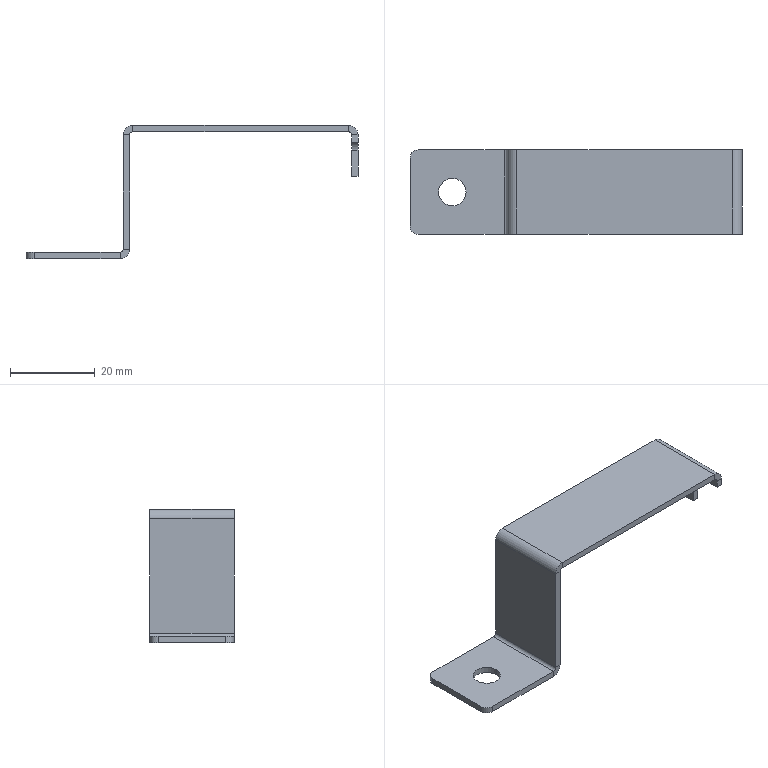Part | STEP file | 10-26 lift limit stopper (Default) | 1 solid | 40 faces | box 78.5 x 20 x 31.5 mm | volume 3271 mm3 | plane 28 | cylinder 12 | commonest cylinder face diameters 4 x4 1.473 x3 4.473 x3 6.5 x2
STEP:
#1=CARTESIAN_POINT('',(-4.75,0.,-1.5));
#2=VERTEX_POINT('',#1);
#3=CARTESIAN_POINT('',(1.75,0.,-1.5));
#4=VERTEX_POINT('',#3);
#5=CARTESIAN_POINT('',(-1.5,0.,-1.5));
#6=DIRECTION('',(0.,0.,1.));
#7=DIRECTION('',(1.,0.,0.));
#8=AXIS2_PLACEMENT_3D('',#5,#6,#7);
#9=CIRCLE('',#8,3.25);
#10=EDGE_CURVE('',#2,#4,#9,.T.);
#11=ORIENTED_EDGE('',*,*,#10,.F.);
#12=CARTESIAN_POINT('',(-4.75,0.,0.));
#13=VERTEX_POINT('',#12);
#14=CARTESIAN_POINT('',(-4.75,0.,-10.));
#15=DIRECTION('',(0.,0.,1.));
#16=VECTOR('',#15,1000.);
#17=LINE('',#14,#16);
#18=EDGE_CURVE('',#2,#13,#17,.T.);
#19=ORIENTED_EDGE('',*,*,#18,.T.);
#20=CARTESIAN_POINT('',(1.75,0.,0.));
#21=VERTEX_POINT('',#20);
#22=CARTESIAN_POINT('',(-1.5,0.,0.));
#23=DIRECTION('',(0.,0.,1.));
#24=DIRECTION('',(1.,0.,0.));
#25=AXIS2_PLACEMENT_3D('',#22,#23,#24);
#26=CIRCLE('',#25,3.25);
#27=EDGE_CURVE('',#13,#21,#26,.T.);
#28=ORIENTED_EDGE('',*,*,#27,.T.);
#29=CARTESIAN_POINT('',(1.75,0.,-10.));
#30=DIRECTION('',(0.,0.,1.));
#31=VECTOR('',#30,1000.);
#32=LINE('',#29,#31);
#33=EDGE_CURVE('',#4,#21,#32,.T.);
#34=ORIENTED_EDGE('',*,*,#33,.F.);
#35=EDGE_LOOP('',(#11,#19,#28,#34));
#36=FACE_OUTER_BOUND('',#35,.T.);
#37=CARTESIAN_POINT('',(-1.5,0.,-10.));
#38=DIRECTION('',(0.,0.,1.));
#39=DIRECTION('',(1.,0.,0.));
#40=AXIS2_PLACEMENT_3D('',#37,#38,#39);
#41=CYLINDRICAL_SURFACE('',#40,3.25);
#42=ADVANCED_FACE('',(#36),#41,.F.);
#43=CARTESIAN_POINT('',(64.763,-10.,28.5));
#44=VERTEX_POINT('',#43);
#45=CARTESIAN_POINT('',(13.737,-10.,28.5));
#46=VERTEX_POINT('',#45);
#47=CARTESIAN_POINT('',(13.,-10.,28.5));
#48=DIRECTION('',(-1.,0.,0.));
#49=VECTOR('',#48,1000.);
#50=LINE('',#47,#49);
#51=EDGE_CURVE('',#44,#46,#50,.T.);
#52=ORIENTED_EDGE('',*,*,#51,.F.);
#53=CARTESIAN_POINT('',(64.763,-10.,30.));
#54=VERTEX_POINT('',#53);
#55=CARTESIAN_POINT('',(64.763,-10.,28.5));
#56=DIRECTION('',(0.,0.,1.));
#57=VECTOR('',#56,1000.);
#58=LINE('',#55,#57);
#59=EDGE_CURVE('',#44,#54,#58,.T.);
#60=ORIENTED_EDGE('',*,*,#59,.T.);
#61=CARTESIAN_POINT('',(13.737,-10.,30.));
#62=VERTEX_POINT('',#61);
#63=CARTESIAN_POINT('',(13.,-10.,30.));
#64=DIRECTION('',(-1.,0.,0.));
#65=VECTOR('',#64,1000.);
#66=LINE('',#63,#65);
#67=EDGE_CURVE('',#54,#62,#66,.T.);
#68=ORIENTED_EDGE('',*,*,#67,.T.);
#69=CARTESIAN_POINT('',(13.737,-10.,28.5));
#70=DIRECTION('',(0.,0.,1.));
#71=VECTOR('',#70,1000.);
#72=LINE('',#69,#71);
#73=EDGE_CURVE('',#46,#62,#72,.T.);
#74=ORIENTED_EDGE('',*,*,#73,.F.);
#75=EDGE_LOOP('',(#52,#60,#68,#74));
#76=FACE_OUTER_BOUND('',#75,.T.);
#77=CARTESIAN_POINT('',(13.,-10.,30.));
#78=DIRECTION('',(0.,-1.,0.));
#79=DIRECTION('',(1.,0.,0.));
#80=AXIS2_PLACEMENT_3D('',#77,#78,#79);
#81=PLANE('',#80);
#82=ADVANCED_FACE('',(#76),#81,.T.);
#83=ORIENTED_EDGE('',*,*,#67,.F.);
#84=CARTESIAN_POINT('',(64.763,10.,30.));
#85=VERTEX_POINT('',#84);
#86=CARTESIAN_POINT('',(64.763,-10.,30.));
#87=DIRECTION('',(0.,1.,0.));
#88=VECTOR('',#87,1000.);
#89=LINE('',#86,#88);
#90=EDGE_CURVE('',#54,#85,#89,.T.);
#91=ORIENTED_EDGE('',*,*,#90,.T.);
#92=CARTESIAN_POINT('',(13.737,10.,30.));
#93=VERTEX_POINT('',#92);
#94=CARTESIAN_POINT('',(65.5,10.,30.));
#95=DIRECTION('',(1.,0.,0.));
#96=VECTOR('',#95,1000.);
#97=LINE('',#94,#96);
#98=EDGE_CURVE('',#93,#85,#97,.T.);
#99=ORIENTED_EDGE('',*,*,#98,.F.);
#100=CARTESIAN_POINT('',(13.737,-10.,30.));
#101=DIRECTION('',(0.,-1.,0.));
#102=VECTOR('',#101,1000.);
#103=LINE('',#100,#102);
#104=EDGE_CURVE('',#93,#62,#103,.T.);
#105=ORIENTED_EDGE('',*,*,#104,.T.);
#106=EDGE_LOOP('',(#83,#91,#99,#105));
#107=FACE_OUTER_BOUND('',#106,.T.);
#108=CARTESIAN_POINT('',(13.,-10.,30.));
#109=DIRECTION('',(0.,0.,1.));
#110=DIRECTION('',(1.,0.,0.));
#111=AXIS2_PLACEMENT_3D('',#108,#109,#110);
#112=PLANE('',#111);
#113=ADVANCED_FACE('',(#107),#112,.T.);
#114=CARTESIAN_POINT('',(64.763,10.,28.5));
#115=VERTEX_POINT('',#114);
#116=CARTESIAN_POINT('',(64.763,-10.,28.5));
#117=DIRECTION('',(0.,1.,0.));
#118=VECTOR('',#117,1000.);
#119=LINE('',#116,#118);
#120=EDGE_CURVE('',#44,#115,#119,.T.);
#121=ORIENTED_EDGE('',*,*,#120,.F.);
#122=ORIENTED_EDGE('',*,*,#51,.T.);
#123=CARTESIAN_POINT('',(13.737,10.,28.5));
#124=VERTEX_POINT('',#123);
#125=CARTESIAN_POINT('',(13.737,10.,28.5));
#126=DIRECTION('',(0.,-1.,0.));
#127=VECTOR('',#126,1000.);
#128=LINE('',#125,#127);
#129=EDGE_CURVE('',#124,#46,#128,.T.);
#130=ORIENTED_EDGE('',*,*,#129,.F.);
#131=CARTESIAN_POINT('',(65.5,10.,28.5));
#132=DIRECTION('',(1.,0.,0.));
#133=VECTOR('',#132,1000.);
#134=LINE('',#131,#133);
#135=EDGE_CURVE('',#124,#115,#134,.T.);
#136=ORIENTED_EDGE('',*,*,#135,.T.);
#137=EDGE_LOOP('',(#121,#122,#130,#136));
#138=FACE_OUTER_BOUND('',#137,.T.);
#139=CARTESIAN_POINT('',(13.,-10.,28.5));
#140=DIRECTION('',(0.,0.,1.));
#141=DIRECTION('',(1.,0.,0.));
#142=AXIS2_PLACEMENT_3D('',#139,#140,#141);
#143=PLANE('',#142);
#144=ADVANCED_FACE('',(#138),#143,.F.);
#145=CARTESIAN_POINT('',(13.,-10.,0.7366));
#146=VERTEX_POINT('',#145);
#147=CARTESIAN_POINT('',(13.,-10.,27.763));
#148=VERTEX_POINT('',#147);
#149=CARTESIAN_POINT('',(13.,-10.,28.5));
#150=DIRECTION('',(0.,0.,1.));
#151=VECTOR('',#150,1000.);
#152=LINE('',#149,#151);
#153=EDGE_CURVE('',#146,#148,#152,.T.);
#154=ORIENTED_EDGE('',*,*,#153,.T.);
#155=CARTESIAN_POINT('',(11.5,-10.,27.763));
#156=VERTEX_POINT('',#155);
#157=CARTESIAN_POINT('',(13.,-10.,27.763));
#158=DIRECTION('',(-1.,0.,0.));
#159=VECTOR('',#158,1000.);
#160=LINE('',#157,#159);
#161=EDGE_CURVE('',#148,#156,#160,.T.);
#162=ORIENTED_EDGE('',*,*,#161,.T.);
#163=CARTESIAN_POINT('',(11.5,-10.,0.7366));
#164=VERTEX_POINT('',#163);
#165=CARTESIAN_POINT('',(11.5,-10.,28.5));
#166=DIRECTION('',(0.,0.,1.));
#167=VECTOR('',#166,1000.);
#168=LINE('',#165,#167);
#169=EDGE_CURVE('',#164,#156,#168,.T.);
#170=ORIENTED_EDGE('',*,*,#169,.F.);
#171=CARTESIAN_POINT('',(11.5,-10.,0.7366));
#172=DIRECTION('',(1.,0.,0.));
#173=VECTOR('',#172,1000.);
#174=LINE('',#171,#173);
#175=EDGE_CURVE('',#164,#146,#174,.T.);
#176=ORIENTED_EDGE('',*,*,#175,.T.);
#177=EDGE_LOOP('',(#154,#162,#170,#176));
#178=FACE_OUTER_BOUND('',#177,.T.);
#179=CARTESIAN_POINT('',(13.,-10.,28.5));
#180=DIRECTION('',(0.,-1.,0.));
#181=DIRECTION('',(1.,0.,0.));
#182=AXIS2_PLACEMENT_3D('',#179,#180,#181);
#183=PLANE('',#182);
#184=ADVANCED_FACE('',(#178),#183,.T.);
#185=CARTESIAN_POINT('',(13.,10.,27.763));
#186=VERTEX_POINT('',#185);
#187=CARTESIAN_POINT('',(13.,10.,0.7366));
#188=VERTEX_POINT('',#187);
#189=CARTESIAN_POINT('',(13.,10.,0.));
#190=DIRECTION('',(0.,0.,-1.));
#191=VECTOR('',#190,1000.);
#192=LINE('',#189,#191);
#193=EDGE_CURVE('',#186,#188,#192,.T.);
#194=ORIENTED_EDGE('',*,*,#193,.F.);
#195=CARTESIAN_POINT('',(13.,-10.,27.763));
#196=DIRECTION('',(0.,1.,0.));
#197=VECTOR('',#196,1000.);
#198=LINE('',#195,#197);
#199=EDGE_CURVE('',#148,#186,#198,.T.);
#200=ORIENTED_EDGE('',*,*,#199,.F.);
#201=ORIENTED_EDGE('',*,*,#153,.F.);
#202=CARTESIAN_POINT('',(13.,10.,0.7366));
#203=DIRECTION('',(0.,1.,0.));
#204=VECTOR('',#203,1000.);
#205=LINE('',#202,#204);
#206=EDGE_CURVE('',#146,#188,#205,.T.);
#207=ORIENTED_EDGE('',*,*,#206,.T.);
#208=EDGE_LOOP('',(#194,#200,#201,#207));
#209=FACE_OUTER_BOUND('',#208,.T.);
#210=CARTESIAN_POINT('',(13.,10.,0.));
#211=DIRECTION('',(1.,0.,0.));
#212=DIRECTION('',(0.,0.,-1.));
#213=AXIS2_PLACEMENT_3D('',#210,#211,#212);
#214=PLANE('',#213);
#215=ADVANCED_FACE('',(#209),#214,.T.);
#216=CARTESIAN_POINT('',(11.5,10.,27.763));
#217=VERTEX_POINT('',#216);
#218=CARTESIAN_POINT('',(11.5,-10.,27.763));
#219=DIRECTION('',(0.,1.,0.));
#220=VECTOR('',#219,1000.);
#221=LINE('',#218,#220);
#222=EDGE_CURVE('',#156,#217,#221,.T.);
#223=ORIENTED_EDGE('',*,*,#222,.T.);
#224=CARTESIAN_POINT('',(11.5,10.,0.7366));
#225=VERTEX_POINT('',#224);
#226=CARTESIAN_POINT('',(11.5,10.,0.));
#227=DIRECTION('',(0.,0.,-1.));
#228=VECTOR('',#227,1000.);
#229=LINE('',#226,#228);
#230=EDGE_CURVE('',#217,#225,#229,.T.);
#231=ORIENTED_EDGE('',*,*,#230,.T.);
#232=CARTESIAN_POINT('',(11.5,-10.,0.7366));
#233=DIRECTION('',(0.,1.,0.));
#234=VECTOR('',#233,1000.);
#235=LINE('',#232,#234);
#236=EDGE_CURVE('',#164,#225,#235,.T.);
#237=ORIENTED_EDGE('',*,*,#236,.F.);
#238=ORIENTED_EDGE('',*,*,#169,.T.);
#239=EDGE_LOOP('',(#223,#231,#237,#238));
#240=FACE_OUTER_BOUND('',#239,.T.);
#241=CARTESIAN_POINT('',(11.5,10.,0.));
#242=DIRECTION('',(1.,0.,0.));
#243=DIRECTION('',(0.,0.,-1.));
#244=AXIS2_PLACEMENT_3D('',#241,#242,#243);
#245=PLANE('',#244);
#246=ADVANCED_FACE('',(#240),#245,.F.);
#247=CARTESIAN_POINT('',(10.763,10.,-1.5));
#248=VERTEX_POINT('',#247);
#249=CARTESIAN_POINT('',(-9.5,10.,-1.5));
#250=VERTEX_POINT('',#249);
#251=CARTESIAN_POINT('',(-11.5,10.,-1.5));
#252=DIRECTION('',(-1.,0.,0.));
#253=VECTOR('',#252,1000.);
#254=LINE('',#251,#253);
#255=EDGE_CURVE('',#248,#250,#254,.T.);
#256=ORIENTED_EDGE('',*,*,#255,.T.);
#257=CARTESIAN_POINT('',(-9.5,10.,0.));
#258=VERTEX_POINT('',#257);
#259=CARTESIAN_POINT('',(-9.5,10.,-1.5));
#260=DIRECTION('',(0.,0.,1.));
#261=VECTOR('',#260,1000.);
#262=LINE('',#259,#261);
#263=EDGE_CURVE('',#250,#258,#262,.T.);
#264=ORIENTED_EDGE('',*,*,#263,.T.);
#265=CARTESIAN_POINT('',(10.763,10.,0.));
#266=VERTEX_POINT('',#265);
#267=CARTESIAN_POINT('',(-11.5,10.,0.));
#268=DIRECTION('',(-1.,0.,0.));
#269=VECTOR('',#268,1000.);
#270=LINE('',#267,#269);
#271=EDGE_CURVE('',#266,#258,#270,.T.);
#272=ORIENTED_EDGE('',*,*,#271,.F.);
#273=CARTESIAN_POINT('',(10.763,10.,0.));
#274=DIRECTION('',(0.,0.,-1.));
#275=VECTOR('',#274,1000.);
#276=LINE('',#273,#275);
#277=EDGE_CURVE('',#266,#248,#276,.T.);
#278=ORIENTED_EDGE('',*,*,#277,.T.);
#279=EDGE_LOOP('',(#256,#264,#272,#278));
#280=FACE_OUTER_BOUND('',#279,.T.);
#281=CARTESIAN_POINT('',(-11.5,10.,-1.5));
#282=DIRECTION('',(0.,1.,0.));
#283=DIRECTION('',(0.,0.,1.));
#284=AXIS2_PLACEMENT_3D('',#281,#282,#283);
#285=PLANE('',#284);
#286=ADVANCED_FACE('',(#280),#285,.T.);
#287=CARTESIAN_POINT('',(-1.5,0.,-1.5));
#288=DIRECTION('',(0.,0.,1.));
#289=DIRECTION('',(1.,0.,0.));
#290=AXIS2_PLACEMENT_3D('',#287,#288,#289);
#291=CIRCLE('',#290,3.25);
#292=EDGE_CURVE('',#4,#2,#291,.T.);
#293=ORIENTED_EDGE('',*,*,#292,.T.);
#294=ORIENTED_EDGE('',*,*,#10,.T.);
#295=EDGE_LOOP('',(#293,#294));
#296=FACE_BOUND('',#295,.T.);
#297=CARTESIAN_POINT('',(-9.5,-10.,-1.5));
#298=VERTEX_POINT('',#297);
#299=CARTESIAN_POINT('',(10.763,-10.,-1.5));
#300=VERTEX_POINT('',#299);
#301=CARTESIAN_POINT('',(-11.5,-10.,-1.5));
#302=DIRECTION('',(1.,0.,0.));
#303=VECTOR('',#302,1000.);
#304=LINE('',#301,#303);
#305=EDGE_CURVE('',#298,#300,#304,.T.);
#306=ORIENTED_EDGE('',*,*,#305,.F.);
#307=CARTESIAN_POINT('',(-11.5,-8.,-1.5));
#308=VERTEX_POINT('',#307);
#309=CARTESIAN_POINT('',(-9.5,-8.,-1.5));
#310=DIRECTION('',(0.,0.,-1.));
#311=DIRECTION('',(1.,0.,0.));
#312=AXIS2_PLACEMENT_3D('',#309,#310,#311);
#313=CIRCLE('',#312,2.);
#314=EDGE_CURVE('',#298,#308,#313,.T.);
#315=ORIENTED_EDGE('',*,*,#314,.T.);
#316=CARTESIAN_POINT('',(-11.5,8.,-1.5));
#317=VERTEX_POINT('',#316);
#318=CARTESIAN_POINT('',(-11.5,10.,-1.5));
#319=DIRECTION('',(0.,-1.,0.));
#320=VECTOR('',#319,1000.);
#321=LINE('',#318,#320);
#322=EDGE_CURVE('',#317,#308,#321,.T.);
#323=ORIENTED_EDGE('',*,*,#322,.F.);
#324=CARTESIAN_POINT('',(-9.5,8.,-1.5));
#325=DIRECTION('',(0.,0.,-1.));
#326=DIRECTION('',(1.,0.,0.));
#327=AXIS2_PLACEMENT_3D('',#324,#325,#326);
#328=CIRCLE('',#327,2.);
#329=EDGE_CURVE('',#317,#250,#328,.T.);
#330=ORIENTED_EDGE('',*,*,#329,.T.);
#331=ORIENTED_EDGE('',*,*,#255,.F.);
#332=CARTESIAN_POINT('',(10.763,10.,-1.5));
#333=DIRECTION('',(0.,-1.,0.));
#334=VECTOR('',#333,1000.);
#335=LINE('',#332,#334);
#336=EDGE_CURVE('',#248,#300,#335,.T.);
#337=ORIENTED_EDGE('',*,*,#336,.T.);
#338=EDGE_LOOP('',(#306,#315,#323,#330,#331,#337));
#339=FACE_OUTER_BOUND('',#338,.T.);
#340=CARTESIAN_POINT('',(11.5,-10.,-1.5));
#341=DIRECTION('',(0.,0.,1.));
#342=DIRECTION('',(1.,0.,0.));
#343=AXIS2_PLACEMENT_3D('',#340,#341,#342);
#344=PLANE('',#343);
#345=ADVANCED_FACE('',(#296,#339),#344,.F.);
#346=CARTESIAN_POINT('',(-1.5,0.,0.));
#347=DIRECTION('',(0.,0.,1.));
#348=DIRECTION('',(1.,0.,0.));
#349=AXIS2_PLACEMENT_3D('',#346,#347,#348);
#350=CIRCLE('',#349,3.25);
#351=EDGE_CURVE('',#21,#13,#350,.T.);
#352=ORIENTED_EDGE('',*,*,#351,.F.);
#353=ORIENTED_EDGE('',*,*,#27,.F.);
#354=EDGE_LOOP('',(#352,#353));
#355=FACE_BOUND('',#354,.T.);
#356=CARTESIAN_POINT('',(-11.5,8.,0.));
#357=VERTEX_POINT('',#356);
#358=CARTESIAN_POINT('',(-11.5,-8.,0.));
#359=VERTEX_POINT('',#358);
#360=CARTESIAN_POINT('',(-11.5,10.,0.));
#361=DIRECTION('',(0.,-1.,0.));
#362=VECTOR('',#361,1000.);
#363=LINE('',#360,#362);
#364=EDGE_CURVE('',#357,#359,#363,.T.);
#365=ORIENTED_EDGE('',*,*,#364,.T.);
#366=CARTESIAN_POINT('',(-9.5,-10.,0.));
#367=VERTEX_POINT('',#366);
#368=CARTESIAN_POINT('',(-9.5,-8.,0.));
#369=DIRECTION('',(0.,0.,1.));
#370=DIRECTION('',(1.,0.,0.));
#371=AXIS2_PLACEMENT_3D('',#368,#369,#370);
#372=CIRCLE('',#371,2.);
#373=EDGE_CURVE('',#359,#367,#372,.T.);
#374=ORIENTED_EDGE('',*,*,#373,.T.);
#375=CARTESIAN_POINT('',(10.763,-10.,0.));
#376=VERTEX_POINT('',#375);
#377=CARTESIAN_POINT('',(-11.5,-10.,0.));
#378=DIRECTION('',(1.,0.,0.));
#379=VECTOR('',#378,1000.);
#380=LINE('',#377,#379);
#381=EDGE_CURVE('',#367,#376,#380,.T.);
#382=ORIENTED_EDGE('',*,*,#381,.T.);
#383=CARTESIAN_POINT('',(10.763,10.,0.));
#384=DIRECTION('',(0.,-1.,0.));
#385=VECTOR('',#384,1000.);
#386=LINE('',#383,#385);
#387=EDGE_CURVE('',#266,#376,#386,.T.);
#388=ORIENTED_EDGE('',*,*,#387,.F.);
#389=ORIENTED_EDGE('',*,*,#271,.T.);
#390=CARTESIAN_POINT('',(-9.5,8.,0.));
#391=DIRECTION('',(0.,0.,1.));
#392=DIRECTION('',(1.,0.,0.));
#393=AXIS2_PLACEMENT_3D('',#390,#391,#392);
#394=CIRCLE('',#393,2.);
#395=EDGE_CURVE('',#258,#357,#394,.T.);
#396=ORIENTED_EDGE('',*,*,#395,.T.);
#397=EDGE_LOOP('',(#365,#374,#382,#388,#389,#396));
#398=FACE_OUTER_BOUND('',#397,.T.);
#399=CARTESIAN_POINT('',(11.5,-10.,0.));
#400=DIRECTION('',(0.,0.,1.));
#401=DIRECTION('',(1.,0.,0.));
#402=AXIS2_PLACEMENT_3D('',#399,#400,#401);
#403=PLANE('',#402);
#404=ADVANCED_FACE('',(#355,#398),#403,.T.);
#405=ORIENTED_EDGE('',*,*,#381,.F.);
#406=CARTESIAN_POINT('',(-9.5,-10.,-1.5));
#407=DIRECTION('',(0.,0.,-1.));
#408=VECTOR('',#407,1000.);
#409=LINE('',#406,#408);
#410=EDGE_CURVE('',#367,#298,#409,.T.);
#411=ORIENTED_EDGE('',*,*,#410,.T.);
#412=ORIENTED_EDGE('',*,*,#305,.T.);
#413=CARTESIAN_POINT('',(10.763,-10.,0.));
#414=DIRECTION('',(0.,0.,-1.));
#415=VECTOR('',#414,1000.);
#416=LINE('',#413,#415);
#417=EDGE_CURVE('',#376,#300,#416,.T.);
#418=ORIENTED_EDGE('',*,*,#417,.F.);
#419=EDGE_LOOP('',(#405,#411,#412,#418));
#420=FACE_OUTER_BOUND('',#419,.T.);
#421=CARTESIAN_POINT('',(-11.5,-10.,-1.5));
#422=DIRECTION('',(0.,-1.,0.));
#423=DIRECTION('',(0.,0.,-1.));
#424=AXIS2_PLACEMENT_3D('',#421,#422,#423);
#425=PLANE('',#424);
#426=ADVANCED_FACE('',(#420),#425,.T.);
#427=ORIENTED_EDGE('',*,*,#322,.T.);
#428=CARTESIAN_POINT('',(-11.5,-8.,-1.5));
#429=DIRECTION('',(0.,0.,1.));
#430=VECTOR('',#429,1000.);
#431=LINE('',#428,#430);
#432=EDGE_CURVE('',#308,#359,#431,.T.);
#433=ORIENTED_EDGE('',*,*,#432,.T.);
#434=ORIENTED_EDGE('',*,*,#364,.F.);
#435=CARTESIAN_POINT('',(-11.5,8.,-1.5));
#436=DIRECTION('',(0.,0.,-1.));
#437=VECTOR('',#436,1000.);
#438=LINE('',#435,#437);
#439=EDGE_CURVE('',#357,#317,#438,.T.);
#440=ORIENTED_EDGE('',*,*,#439,.T.);
#441=EDGE_LOOP('',(#427,#433,#434,#440));
#442=FACE_OUTER_BOUND('',#441,.T.);
#443=CARTESIAN_POINT('',(-11.5,10.,-1.5));
#444=DIRECTION('',(-1.,0.,0.));
#445=DIRECTION('',(0.,0.,1.));
#446=AXIS2_PLACEMENT_3D('',#443,#444,#445);
#447=PLANE('',#446);
#448=ADVANCED_FACE('',(#442),#447,.T.);
#449=ORIENTED_EDGE('',*,*,#175,.F.);
#450=CARTESIAN_POINT('',(10.763,-10.,0.7366));
#451=DIRECTION('',(0.,-1.,0.));
#452=DIRECTION('',(0.,0.,1.));
#453=AXIS2_PLACEMENT_3D('',#450,#451,#452);
#454=CIRCLE('',#453,0.7366);
#455=EDGE_CURVE('',#376,#164,#454,.T.);
#456=ORIENTED_EDGE('',*,*,#455,.F.);
#457=ORIENTED_EDGE('',*,*,#417,.T.);
#458=CARTESIAN_POINT('',(10.763,-10.,0.7366));
#459=DIRECTION('',(0.,-1.,0.));
#460=DIRECTION('',(0.,0.,1.));
#461=AXIS2_PLACEMENT_3D('',#458,#459,#460);
#462=CIRCLE('',#461,2.237);
#463=EDGE_CURVE('',#300,#146,#462,.T.);
#464=ORIENTED_EDGE('',*,*,#463,.T.);
#465=EDGE_LOOP('',(#449,#456,#457,#464));
#466=FACE_OUTER_BOUND('',#465,.T.);
#467=CARTESIAN_POINT('',(10.763,-10.,0.7366));
#468=DIRECTION('',(0.,-1.,0.));
#469=DIRECTION('',(0.,0.,-1.));
#470=AXIS2_PLACEMENT_3D('',#467,#468,#469);
#471=PLANE('',#470);
#472=ADVANCED_FACE('',(#466),#471,.T.);
#473=CARTESIAN_POINT('',(10.763,10.,0.7366));
#474=DIRECTION('',(0.,1.,0.));
#475=DIRECTION('',(0.,0.,1.));
#476=AXIS2_PLACEMENT_3D('',#473,#474,#475);
#477=CIRCLE('',#476,0.7366);
#478=EDGE_CURVE('',#225,#266,#477,.T.);
#479=ORIENTED_EDGE('',*,*,#478,.F.);
#480=CARTESIAN_POINT('',(11.5,10.,0.7366));
#481=DIRECTION('',(1.,0.,0.));
#482=VECTOR('',#481,1000.);
#483=LINE('',#480,#482);
#484=EDGE_CURVE('',#225,#188,#483,.T.);
#485=ORIENTED_EDGE('',*,*,#484,.T.);
#486=CARTESIAN_POINT('',(10.763,10.,0.7366));
#487=DIRECTION('',(0.,1.,0.));
#488=DIRECTION('',(0.,0.,1.));
#489=AXIS2_PLACEMENT_3D('',#486,#487,#488);
#490=CIRCLE('',#489,2.237);
#491=EDGE_CURVE('',#188,#248,#490,.T.);
#492=ORIENTED_EDGE('',*,*,#491,.T.);
#493=ORIENTED_EDGE('',*,*,#277,.F.);
#494=EDGE_LOOP('',(#479,#485,#492,#493));
#495=FACE_OUTER_BOUND('',#494,.T.);
#496=CARTESIAN_POINT('',(10.763,10.,0.7366));
#497=DIRECTION('',(0.,-1.,0.));
#498=DIRECTION('',(0.,0.,-1.));
#499=AXIS2_PLACEMENT_3D('',#496,#497,#498);
#500=PLANE('',#499);
#501=ADVANCED_FACE('',(#495),#500,.F.);
#502=ORIENTED_EDGE('',*,*,#336,.F.);
#503=ORIENTED_EDGE('',*,*,#491,.F.);
#504=ORIENTED_EDGE('',*,*,#206,.F.);
#505=ORIENTED_EDGE('',*,*,#463,.F.);
#506=EDGE_LOOP('',(#502,#503,#504,#505));
#507=FACE_OUTER_BOUND('',#506,.T.);
#508=CARTESIAN_POINT('',(10.763,10.,0.7366));
#509=DIRECTION('',(0.,1.,0.));
#510=DIRECTION('',(1.,0.,0.));
#511=AXIS2_PLACEMENT_3D('',#508,#509,#510);
#512=CYLINDRICAL_SURFACE('',#511,2.237);
#513=ADVANCED_FACE('',(#507),#512,.T.);
#514=ORIENTED_EDGE('',*,*,#387,.T.);
#515=ORIENTED_EDGE('',*,*,#455,.T.);
#516=ORIENTED_EDGE('',*,*,#236,.T.);
#517=ORIENTED_EDGE('',*,*,#478,.T.);
#518=EDGE_LOOP('',(#514,#515,#516,#517));
#519=FACE_OUTER_BOUND('',#518,.T.);
#520=CARTESIAN_POINT('',(10.763,10.,0.7366));
#521=DIRECTION('',(0.,1.,0.));
#522=DIRECTION('',(1.,0.,0.));
#523=AXIS2_PLACEMENT_3D('',#520,#521,#522);
#524=CYLINDRICAL_SURFACE('',#523,0.7366);
#525=ADVANCED_FACE('',(#519),#524,.F.);
#526=CARTESIAN_POINT('',(13.,10.,27.763));
#527=DIRECTION('',(-1.,0.,0.));
#528=VECTOR('',#527,1000.);
#529=LINE('',#526,#528);
#530=EDGE_CURVE('',#186,#217,#529,.T.);
#531=ORIENTED_EDGE('',*,*,#530,.F.);
#532=ORIENTED_EDGE('',*,*,#193,.T.);
#533=ORIENTED_EDGE('',*,*,#484,.F.);
#534=ORIENTED_EDGE('',*,*,#230,.F.);
#535=EDGE_LOOP('',(#531,#532,#533,#534));
#536=FACE_OUTER_BOUND('',#535,.T.);
#537=CARTESIAN_POINT('',(13.,10.,0.));
#538=DIRECTION('',(0.,1.,0.));
#539=DIRECTION('',(-1.,0.,0.));
#540=AXIS2_PLACEMENT_3D('',#537,#538,#539);
#541=PLANE('',#540);
#542=ADVANCED_FACE('',(#536),#541,.T.);
#543=CARTESIAN_POINT('',(13.737,10.,28.5));
#544=DIRECTION('',(0.,0.,1.));
#545=VECTOR('',#544,1000.);
#546=LINE('',#543,#545);
#547=EDGE_CURVE('',#124,#93,#546,.T.);
#548=ORIENTED_EDGE('',*,*,#547,.F.);
#549=CARTESIAN_POINT('',(13.737,10.,27.763));
#550=DIRECTION('',(0.,1.,0.));
#551=DIRECTION('',(0.,0.,-1.));
#552=AXIS2_PLACEMENT_3D('',#549,#550,#551);
#553=CIRCLE('',#552,0.7366);
#554=EDGE_CURVE('',#186,#124,#553,.T.);
#555=ORIENTED_EDGE('',*,*,#554,.F.);
#556=ORIENTED_EDGE('',*,*,#530,.T.);
#557=CARTESIAN_POINT('',(13.737,10.,27.763));
#558=DIRECTION('',(0.,1.,0.));
#559=DIRECTION('',(0.,0.,-1.));
#560=AXIS2_PLACEMENT_3D('',#557,#558,#559);
#561=CIRCLE('',#560,2.237);
#562=EDGE_CURVE('',#217,#93,#561,.T.);
#563=ORIENTED_EDGE('',*,*,#562,.T.);
#564=EDGE_LOOP('',(#548,#555,#556,#563));
#565=FACE_OUTER_BOUND('',#564,.T.);
#566=CARTESIAN_POINT('',(13.737,10.,27.763));
#567=DIRECTION('',(0.,1.,0.));
#568=DIRECTION('',(0.,0.,1.));
#569=AXIS2_PLACEMENT_3D('',#566,#567,#568);
#570=PLANE('',#569);
#571=ADVANCED_FACE('',(#565),#570,.T.);
#572=CARTESIAN_POINT('',(13.737,-10.,27.763));
#573=DIRECTION('',(0.,-1.,0.));
#574=DIRECTION('',(0.,0.,-1.));
#575=AXIS2_PLACEMENT_3D('',#572,#573,#574);
#576=CIRCLE('',#575,0.7366);
#577=EDGE_CURVE('',#46,#148,#576,.T.);
#578=ORIENTED_EDGE('',*,*,#577,.F.);
#579=ORIENTED_EDGE('',*,*,#73,.T.);
#580=CARTESIAN_POINT('',(13.737,-10.,27.763));
#581=DIRECTION('',(0.,-1.,0.));
#582=DIRECTION('',(0.,0.,-1.));
#583=AXIS2_PLACEMENT_3D('',#580,#581,#582);
#584=CIRCLE('',#583,2.237);
#585=EDGE_CURVE('',#62,#156,#584,.T.);
#586=ORIENTED_EDGE('',*,*,#585,.T.);
#587=ORIENTED_EDGE('',*,*,#161,.F.);
#588=EDGE_LOOP('',(#578,#579,#586,#587));
#589=FACE_OUTER_BOUND('',#588,.T.);
#590=CARTESIAN_POINT('',(13.737,-10.,27.763));
#591=DIRECTION('',(0.,1.,0.));
#592=DIRECTION('',(0.,0.,1.));
#593=AXIS2_PLACEMENT_3D('',#590,#591,#592);
#594=PLANE('',#593);
#595=ADVANCED_FACE('',(#589),#594,.F.);
#596=ORIENTED_EDGE('',*,*,#222,.F.);
#597=ORIENTED_EDGE('',*,*,#585,.F.);
#598=ORIENTED_EDGE('',*,*,#104,.F.);
#599=ORIENTED_EDGE('',*,*,#562,.F.);
#600=EDGE_LOOP('',(#596,#597,#598,#599));
#601=FACE_OUTER_BOUND('',#600,.T.);
#602=CARTESIAN_POINT('',(13.737,-10.,27.763));
#603=DIRECTION('',(0.,-1.,0.));
#604=DIRECTION('',(0.,0.,1.));
#605=AXIS2_PLACEMENT_3D('',#602,#603,#604);
#606=CYLINDRICAL_SURFACE('',#605,2.237);
#607=ADVANCED_FACE('',(#601),#606,.T.);
#608=ORIENTED_EDGE('',*,*,#199,.T.);
#609=ORIENTED_EDGE('',*,*,#554,.T.);
#610=ORIENTED_EDGE('',*,*,#129,.T.);
#611=ORIENTED_EDGE('',*,*,#577,.T.);
#612=EDGE_LOOP('',(#608,#609,#610,#611));
#613=FACE_OUTER_BOUND('',#612,.T.);
#614=CARTESIAN_POINT('',(13.737,-10.,27.763));
#615=DIRECTION('',(0.,-1.,0.));
#616=DIRECTION('',(0.,0.,1.));
#617=AXIS2_PLACEMENT_3D('',#614,#615,#616);
#618=CYLINDRICAL_SURFACE('',#617,0.7366);
#619=ADVANCED_FACE('',(#613),#618,.F.);
#620=CARTESIAN_POINT('',(64.763,10.,28.5));
#621=DIRECTION('',(0.,0.,1.));
#622=VECTOR('',#621,1000.);
#623=LINE('',#620,#622);
#624=EDGE_CURVE('',#115,#85,#623,.T.);
#625=ORIENTED_EDGE('',*,*,#624,.F.);
#626=ORIENTED_EDGE('',*,*,#135,.F.);
#627=ORIENTED_EDGE('',*,*,#547,.T.);
#628=ORIENTED_EDGE('',*,*,#98,.T.);
#629=EDGE_LOOP('',(#625,#626,#627,#628));
#630=FACE_OUTER_BOUND('',#629,.T.);
#631=CARTESIAN_POINT('',(65.5,10.,30.));
#632=DIRECTION('',(0.,1.,0.));
#633=DIRECTION('',(-1.,0.,0.));
#634=AXIS2_PLACEMENT_3D('',#631,#632,#633);
#635=PLANE('',#634);
#636=ADVANCED_FACE('',(#630),#635,.T.);
#637=CARTESIAN_POINT('',(65.5,10.,27.763));
#638=VERTEX_POINT('',#637);
#639=CARTESIAN_POINT('',(67.,10.,27.763));
#640=VERTEX_POINT('',#639);
#641=CARTESIAN_POINT('',(65.5,10.,27.763));
#642=DIRECTION('',(1.,0.,0.));
#643=VECTOR('',#642,1000.);
#644=LINE('',#641,#643);
#645=EDGE_CURVE('',#638,#640,#644,.T.);
#646=ORIENTED_EDGE('',*,*,#645,.F.);
#647=CARTESIAN_POINT('',(64.763,10.,27.763));
#648=DIRECTION('',(0.,1.,0.));
#649=DIRECTION('',(0.,0.,-1.));
#650=AXIS2_PLACEMENT_3D('',#647,#648,#649);
#651=CIRCLE('',#650,0.7366);
#652=EDGE_CURVE('',#115,#638,#651,.T.);
#653=ORIENTED_EDGE('',*,*,#652,.F.);
#654=ORIENTED_EDGE('',*,*,#624,.T.);
#655=CARTESIAN_POINT('',(64.763,10.,27.763));
#656=DIRECTION('',(0.,1.,0.));
#657=DIRECTION('',(0.,0.,-1.));
#658=AXIS2_PLACEMENT_3D('',#655,#656,#657);
#659=CIRCLE('',#658,2.237);
#660=EDGE_CURVE('',#85,#640,#659,.T.);
#661=ORIENTED_EDGE('',*,*,#660,.T.);
#662=EDGE_LOOP('',(#646,#653,#654,#661));
#663=FACE_OUTER_BOUND('',#662,.T.);
#664=CARTESIAN_POINT('',(64.763,10.,27.763));
#665=DIRECTION('',(0.,1.,0.));
#666=DIRECTION('',(0.,0.,1.));
#667=AXIS2_PLACEMENT_3D('',#664,#665,#666);
#668=PLANE('',#667);
#669=ADVANCED_FACE('',(#663),#668,.T.);
#670=CARTESIAN_POINT('',(65.5,-10.,27.763));
#671=VERTEX_POINT('',#670);
#672=CARTESIAN_POINT('',(64.763,-10.,27.763));
#673=DIRECTION('',(0.,-1.,0.));
#674=DIRECTION('',(0.,0.,-1.));
#675=AXIS2_PLACEMENT_3D('',#672,#673,#674);
#676=CIRCLE('',#675,0.7366);
#677=EDGE_CURVE('',#671,#44,#676,.T.);
#678=ORIENTED_EDGE('',*,*,#677,.F.);
#679=CARTESIAN_POINT('',(67.,-10.,27.763));
#680=VERTEX_POINT('',#679);
#681=CARTESIAN_POINT('',(65.5,-10.,27.763));
#682=DIRECTION('',(1.,0.,0.));
#683=VECTOR('',#682,1000.);
#684=LINE('',#681,#683);
#685=EDGE_CURVE('',#671,#680,#684,.T.);
#686=ORIENTED_EDGE('',*,*,#685,.T.);
#687=CARTESIAN_POINT('',(64.763,-10.,27.763));
#688=DIRECTION('',(0.,-1.,0.));
#689=DIRECTION('',(0.,0.,-1.));
#690=AXIS2_PLACEMENT_3D('',#687,#688,#689);
#691=CIRCLE('',#690,2.237);
#692=EDGE_CURVE('',#680,#54,#691,.T.);
#693=ORIENTED_EDGE('',*,*,#692,.T.);
#694=ORIENTED_EDGE('',*,*,#59,.F.);
#695=EDGE_LOOP('',(#678,#686,#693,#694));
#696=FACE_OUTER_BOUND('',#695,.T.);
#697=CARTESIAN_POINT('',(64.763,-10.,27.763));
#698=DIRECTION('',(0.,1.,0.));
#699=DIRECTION('',(0.,0.,1.));
#700=AXIS2_PLACEMENT_3D('',#697,#698,#699);
#701=PLANE('',#700);
#702=ADVANCED_FACE('',(#696),#701,.F.);
#703=ORIENTED_EDGE('',*,*,#90,.F.);
#704=ORIENTED_EDGE('',*,*,#692,.F.);
#705=CARTESIAN_POINT('',(67.,-10.,27.763));
#706=DIRECTION('',(0.,-1.,0.));
#707=VECTOR('',#706,1000.);
#708=LINE('',#705,#707);
#709=EDGE_CURVE('',#640,#680,#708,.T.);
#710=ORIENTED_EDGE('',*,*,#709,.F.);
#711=ORIENTED_EDGE('',*,*,#660,.F.);
#712=EDGE_LOOP('',(#703,#704,#710,#711));
#713=FACE_OUTER_BOUND('',#712,.T.);
#714=CARTESIAN_POINT('',(64.763,-10.,27.763));
#715=DIRECTION('',(0.,-1.,0.));
#716=DIRECTION('',(1.,0.,0.));
#717=AXIS2_PLACEMENT_3D('',#714,#715,#716);
#718=CYLINDRICAL_SURFACE('',#717,2.237);
#719=ADVANCED_FACE('',(#713),#718,.T.);
#720=ORIENTED_EDGE('',*,*,#120,.T.);
#721=ORIENTED_EDGE('',*,*,#652,.T.);
#722=CARTESIAN_POINT('',(65.5,10.,27.763));
#723=DIRECTION('',(0.,-1.,0.));
#724=VECTOR('',#723,1000.);
#725=LINE('',#722,#724);
#726=EDGE_CURVE('',#638,#671,#725,.T.);
#727=ORIENTED_EDGE('',*,*,#726,.T.);
#728=ORIENTED_EDGE('',*,*,#677,.T.);
#729=EDGE_LOOP('',(#720,#721,#727,#728));
#730=FACE_OUTER_BOUND('',#729,.T.);
#731=CARTESIAN_POINT('',(64.763,-10.,27.763));
#732=DIRECTION('',(0.,-1.,0.));
#733=DIRECTION('',(1.,0.,0.));
#734=AXIS2_PLACEMENT_3D('',#731,#732,#733);
#735=CYLINDRICAL_SURFACE('',#734,0.7366);
#736=ADVANCED_FACE('',(#730),#735,.F.);
#737=CARTESIAN_POINT('',(65.5,-10.,26.));
#738=VERTEX_POINT('',#737);
#739=CARTESIAN_POINT('',(67.,-10.,26.));
#740=VERTEX_POINT('',#739);
#741=CARTESIAN_POINT('',(57.,-10.,26.));
#742=DIRECTION('',(1.,0.,0.));
#743=VECTOR('',#742,1000.);
#744=LINE('',#741,#743);
#745=EDGE_CURVE('',#738,#740,#744,.T.);
#746=ORIENTED_EDGE('',*,*,#745,.T.);
#747=CARTESIAN_POINT('',(67.,-10.,28.5));
#748=DIRECTION('',(0.,0.,1.));
#749=VECTOR('',#748,1000.);
#750=LINE('',#747,#749);
#751=EDGE_CURVE('',#740,#680,#750,.T.);
#752=ORIENTED_EDGE('',*,*,#751,.T.);
#753=ORIENTED_EDGE('',*,*,#685,.F.);
#754=CARTESIAN_POINT('',(65.5,-10.,28.5));
#755=DIRECTION('',(0.,0.,1.));
#756=VECTOR('',#755,1000.);
#757=LINE('',#754,#756);
#758=EDGE_CURVE('',#738,#671,#757,.T.);
#759=ORIENTED_EDGE('',*,*,#758,.F.);
#760=EDGE_LOOP('',(#746,#752,#753,#759));
#761=FACE_OUTER_BOUND('',#760,.T.);
#762=CARTESIAN_POINT('',(67.,-10.,28.5));
#763=DIRECTION('',(0.,-1.,0.));
#764=DIRECTION('',(0.,0.,-1.));
#765=AXIS2_PLACEMENT_3D('',#762,#763,#764);
#766=PLANE('',#765);
#767=ADVANCED_FACE('',(#761),#766,.T.);
#768=CARTESIAN_POINT('',(65.5,10.,26.));
#769=VERTEX_POINT('',#768);
#770=CARTESIAN_POINT('',(67.,10.,26.));
#771=VERTEX_POINT('',#770);
#772=CARTESIAN_POINT('',(57.,10.,26.));
#773=DIRECTION('',(1.,0.,0.));
#774=VECTOR('',#773,1000.);
#775=LINE('',#772,#774);
#776=EDGE_CURVE('',#769,#771,#775,.T.);
#777=ORIENTED_EDGE('',*,*,#776,.F.);
#778=CARTESIAN_POINT('',(65.5,10.,18.));
#779=DIRECTION('',(0.,0.,-1.));
#780=VECTOR('',#779,1000.);
#781=LINE('',#778,#780);
#782=EDGE_CURVE('',#638,#769,#781,.T.);
#783=ORIENTED_EDGE('',*,*,#782,.F.);
#784=ORIENTED_EDGE('',*,*,#645,.T.);
#785=CARTESIAN_POINT('',(67.,10.,18.));
#786=DIRECTION('',(0.,0.,-1.));
#787=VECTOR('',#786,1000.);
#788=LINE('',#785,#787);
#789=EDGE_CURVE('',#640,#771,#788,.T.);
#790=ORIENTED_EDGE('',*,*,#789,.T.);
#791=EDGE_LOOP('',(#777,#783,#784,#790));
#792=FACE_OUTER_BOUND('',#791,.T.);
#793=CARTESIAN_POINT('',(67.,10.,18.));
#794=DIRECTION('',(0.,1.,0.));
#795=DIRECTION('',(0.,0.,1.));
#796=AXIS2_PLACEMENT_3D('',#793,#794,#795);
#797=PLANE('',#796);
#798=ADVANCED_FACE('',(#792),#797,.T.);
#799=CARTESIAN_POINT('',(67.,-4.,26.));
#800=VERTEX_POINT('',#799);
#801=CARTESIAN_POINT('',(67.,-2.,26.));
#802=DIRECTION('',(0.,-1.,0.));
#803=VECTOR('',#802,1000.);
#804=LINE('',#801,#803);
#805=EDGE_CURVE('',#800,#740,#804,.T.);
#806=ORIENTED_EDGE('',*,*,#805,.F.);
#807=CARTESIAN_POINT('',(67.,-2.,24.));
#808=VERTEX_POINT('',#807);
#809=CARTESIAN_POINT('',(67.,-4.,24.));
#810=DIRECTION('',(-1.,0.,0.));
#811=DIRECTION('',(0.,0.,-1.));
#812=AXIS2_PLACEMENT_3D('',#809,#810,#811);
#813=CIRCLE('',#812,2.);
#814=EDGE_CURVE('',#800,#808,#813,.T.);
#815=ORIENTED_EDGE('',*,*,#814,.T.);
#816=CARTESIAN_POINT('',(67.,-2.,18.));
#817=VERTEX_POINT('',#816);
#818=CARTESIAN_POINT('',(67.,-2.,18.));
#819=DIRECTION('',(0.,0.,1.));
#820=VECTOR('',#819,1000.);
#821=LINE('',#818,#820);
#822=EDGE_CURVE('',#817,#808,#821,.T.);
#823=ORIENTED_EDGE('',*,*,#822,.F.);
#824=CARTESIAN_POINT('',(67.,2.,18.));
#825=VERTEX_POINT('',#824);
#826=CARTESIAN_POINT('',(67.,-10.,18.));
#827=DIRECTION('',(0.,-1.,0.));
#828=VECTOR('',#827,1000.);
#829=LINE('',#826,#828);
#830=EDGE_CURVE('',#825,#817,#829,.T.);
#831=ORIENTED_EDGE('',*,*,#830,.F.);
#832=CARTESIAN_POINT('',(67.,2.,24.));
#833=VERTEX_POINT('',#832);
#834=CARTESIAN_POINT('',(67.,2.,26.));
#835=DIRECTION('',(0.,0.,-1.));
#836=VECTOR('',#835,1000.);
#837=LINE('',#834,#836);
#838=EDGE_CURVE('',#833,#825,#837,.T.);
#839=ORIENTED_EDGE('',*,*,#838,.F.);
#840=CARTESIAN_POINT('',(67.,4.,26.));
#841=VERTEX_POINT('',#840);
#842=CARTESIAN_POINT('',(67.,4.,24.));
#843=DIRECTION('',(-1.,0.,0.));
#844=DIRECTION('',(0.,0.,-1.));
#845=AXIS2_PLACEMENT_3D('',#842,#843,#844);
#846=CIRCLE('',#845,2.);
#847=EDGE_CURVE('',#833,#841,#846,.T.);
#848=ORIENTED_EDGE('',*,*,#847,.T.);
#849=CARTESIAN_POINT('',(67.,10.,26.));
#850=DIRECTION('',(0.,-1.,0.));
#851=VECTOR('',#850,1000.);
#852=LINE('',#849,#851);
#853=EDGE_CURVE('',#771,#841,#852,.T.);
#854=ORIENTED_EDGE('',*,*,#853,.F.);
#855=ORIENTED_EDGE('',*,*,#789,.F.);
#856=ORIENTED_EDGE('',*,*,#709,.T.);
#857=ORIENTED_EDGE('',*,*,#751,.F.);
#858=EDGE_LOOP('',(#806,#815,#823,#831,#839,#848,#854,#855,#856,#857));
#859=FACE_OUTER_BOUND('',#858,.T.);
#860=CARTESIAN_POINT('',(67.,-10.,28.5));
#861=DIRECTION('',(1.,0.,0.));
#862=DIRECTION('',(0.,0.,-1.));
#863=AXIS2_PLACEMENT_3D('',#860,#861,#862);
#864=PLANE('',#863);
#865=ADVANCED_FACE('',(#859),#864,.T.);
#866=CARTESIAN_POINT('',(65.5,-2.,18.));
#867=VERTEX_POINT('',#866);
#868=CARTESIAN_POINT('',(65.5,-2.,24.));
#869=VERTEX_POINT('',#868);
#870=CARTESIAN_POINT('',(65.5,-2.,28.5));
#871=DIRECTION('',(0.,0.,1.));
#872=VECTOR('',#871,1000.);
#873=LINE('',#870,#872);
#874=EDGE_CURVE('',#867,#869,#873,.T.);
#875=ORIENTED_EDGE('',*,*,#874,.T.);
#876=CARTESIAN_POINT('',(65.5,-4.,26.));
#877=VERTEX_POINT('',#876);
#878=CARTESIAN_POINT('',(65.5,-4.,24.));
#879=DIRECTION('',(1.,0.,0.));
#880=DIRECTION('',(0.,0.,-1.));
#881=AXIS2_PLACEMENT_3D('',#878,#879,#880);
#882=CIRCLE('',#881,2.);
#883=EDGE_CURVE('',#869,#877,#882,.T.);
#884=ORIENTED_EDGE('',*,*,#883,.T.);
#885=CARTESIAN_POINT('',(65.5,-10.,26.));
#886=DIRECTION('',(0.,-1.,0.));
#887=VECTOR('',#886,1000.);
#888=LINE('',#885,#887);
#889=EDGE_CURVE('',#877,#738,#888,.T.);
#890=ORIENTED_EDGE('',*,*,#889,.T.);
#891=ORIENTED_EDGE('',*,*,#758,.T.);
#892=ORIENTED_EDGE('',*,*,#726,.F.);
#893=ORIENTED_EDGE('',*,*,#782,.T.);
#894=CARTESIAN_POINT('',(65.5,4.,26.));
#895=VERTEX_POINT('',#894);
#896=CARTESIAN_POINT('',(65.5,-10.,26.));
#897=DIRECTION('',(0.,-1.,0.));
#898=VECTOR('',#897,1000.);
#899=LINE('',#896,#898);
#900=EDGE_CURVE('',#769,#895,#899,.T.);
#901=ORIENTED_EDGE('',*,*,#900,.T.);
#902=CARTESIAN_POINT('',(65.5,2.,24.));
#903=VERTEX_POINT('',#902);
#904=CARTESIAN_POINT('',(65.5,4.,24.));
#905=DIRECTION('',(1.,0.,0.));
#906=DIRECTION('',(0.,0.,-1.));
#907=AXIS2_PLACEMENT_3D('',#904,#905,#906);
#908=CIRCLE('',#907,2.);
#909=EDGE_CURVE('',#895,#903,#908,.T.);
#910=ORIENTED_EDGE('',*,*,#909,.T.);
#911=CARTESIAN_POINT('',(65.5,2.,18.));
#912=VERTEX_POINT('',#911);
#913=CARTESIAN_POINT('',(65.5,2.,28.5));
#914=DIRECTION('',(0.,0.,-1.));
#915=VECTOR('',#914,1000.);
#916=LINE('',#913,#915);
#917=EDGE_CURVE('',#903,#912,#916,.T.);
#918=ORIENTED_EDGE('',*,*,#917,.T.);
#919=CARTESIAN_POINT('',(65.5,-10.,18.));
#920=DIRECTION('',(0.,-1.,0.));
#921=VECTOR('',#920,1000.);
#922=LINE('',#919,#921);
#923=EDGE_CURVE('',#912,#867,#922,.T.);
#924=ORIENTED_EDGE('',*,*,#923,.T.);
#925=EDGE_LOOP('',(#875,#884,#890,#891,#892,#893,#901,#910,#918,#924));
#926=FACE_OUTER_BOUND('',#925,.T.);
#927=CARTESIAN_POINT('',(65.5,-10.,28.5));
#928=DIRECTION('',(1.,0.,0.));
#929=DIRECTION('',(0.,0.,-1.));
#930=AXIS2_PLACEMENT_3D('',#927,#928,#929);
#931=PLANE('',#930);
#932=ADVANCED_FACE('',(#926),#931,.F.);
#933=CARTESIAN_POINT('',(67.,-2.,18.));
#934=DIRECTION('',(1.,0.,0.));
#935=VECTOR('',#934,1000.);
#936=LINE('',#933,#935);
#937=EDGE_CURVE('',#867,#817,#936,.T.);
#938=ORIENTED_EDGE('',*,*,#937,.F.);
#939=ORIENTED_EDGE('',*,*,#923,.F.);
#940=CARTESIAN_POINT('',(67.,2.,18.));
#941=DIRECTION('',(-1.,0.,0.));
#942=VECTOR('',#941,1000.);
#943=LINE('',#940,#942);
#944=EDGE_CURVE('',#825,#912,#943,.T.);
#945=ORIENTED_EDGE('',*,*,#944,.F.);
#946=ORIENTED_EDGE('',*,*,#830,.T.);
#947=EDGE_LOOP('',(#938,#939,#945,#946));
#948=FACE_OUTER_BOUND('',#947,.T.);
#949=CARTESIAN_POINT('',(67.,-10.,18.));
#950=DIRECTION('',(0.,0.,-1.));
#951=DIRECTION('',(-1.,0.,0.));
#952=AXIS2_PLACEMENT_3D('',#949,#950,#951);
#953=PLANE('',#952);
#954=ADVANCED_FACE('',(#948),#953,.T.);
#955=ORIENTED_EDGE('',*,*,#853,.T.);
#956=CARTESIAN_POINT('',(65.5,4.,26.));
#957=DIRECTION('',(-1.,0.,0.));
#958=VECTOR('',#957,1000.);
#959=LINE('',#956,#958);
#960=EDGE_CURVE('',#841,#895,#959,.T.);
#961=ORIENTED_EDGE('',*,*,#960,.T.);
#962=ORIENTED_EDGE('',*,*,#900,.F.);
#963=ORIENTED_EDGE('',*,*,#776,.T.);
#964=EDGE_LOOP('',(#955,#961,#962,#963));
#965=FACE_OUTER_BOUND('',#964,.T.);
#966=CARTESIAN_POINT('',(57.,10.,26.));
#967=DIRECTION('',(0.,0.,1.));
#968=DIRECTION('',(1.,0.,0.));
#969=AXIS2_PLACEMENT_3D('',#966,#967,#968);
#970=PLANE('',#969);
#971=ADVANCED_FACE('',(#965),#970,.F.);
#972=ORIENTED_EDGE('',*,*,#917,.F.);
#973=CARTESIAN_POINT('',(67.,2.,24.));
#974=DIRECTION('',(1.,0.,0.));
#975=VECTOR('',#974,1000.);
#976=LINE('',#973,#975);
#977=EDGE_CURVE('',#903,#833,#976,.T.);
#978=ORIENTED_EDGE('',*,*,#977,.T.);
#979=ORIENTED_EDGE('',*,*,#838,.T.);
#980=ORIENTED_EDGE('',*,*,#944,.T.);
#981=EDGE_LOOP('',(#972,#978,#979,#980));
#982=FACE_OUTER_BOUND('',#981,.T.);
#983=CARTESIAN_POINT('',(57.,2.,26.));
#984=DIRECTION('',(0.,-1.,0.));
#985=DIRECTION('',(0.,0.,-1.));
#986=AXIS2_PLACEMENT_3D('',#983,#984,#985);
#987=PLANE('',#986);
#988=ADVANCED_FACE('',(#982),#987,.F.);
#989=ORIENTED_EDGE('',*,*,#889,.F.);
#990=CARTESIAN_POINT('',(67.,-4.,26.));
#991=DIRECTION('',(1.,0.,0.));
#992=VECTOR('',#991,1000.);
#993=LINE('',#990,#992);
#994=EDGE_CURVE('',#877,#800,#993,.T.);
#995=ORIENTED_EDGE('',*,*,#994,.T.);
#996=ORIENTED_EDGE('',*,*,#805,.T.);
#997=ORIENTED_EDGE('',*,*,#745,.F.);
#998=EDGE_LOOP('',(#989,#995,#996,#997));
#999=FACE_OUTER_BOUND('',#998,.T.);
#1000=CARTESIAN_POINT('',(57.,-2.,26.));
#1001=DIRECTION('',(0.,0.,1.));
#1002=DIRECTION('',(1.,0.,0.));
#1003=AXIS2_PLACEMENT_3D('',#1000,#1001,#1002);
#1004=PLANE('',#1003);
#1005=ADVANCED_FACE('',(#999),#1004,.F.);
#1006=ORIENTED_EDGE('',*,*,#822,.T.);
#1007=CARTESIAN_POINT('',(65.5,-2.,24.));
#1008=DIRECTION('',(-1.,0.,0.));
#1009=VECTOR('',#1008,1000.);
#1010=LINE('',#1007,#1009);
#1011=EDGE_CURVE('',#808,#869,#1010,.T.);
#1012=ORIENTED_EDGE('',*,*,#1011,.T.);
#1013=ORIENTED_EDGE('',*,*,#874,.F.);
#1014=ORIENTED_EDGE('',*,*,#937,.T.);
#1015=EDGE_LOOP('',(#1006,#1012,#1013,#1014));
#1016=FACE_OUTER_BOUND('',#1015,.T.);
#1017=CARTESIAN_POINT('',(57.,-2.,18.));
#1018=DIRECTION('',(0.,1.,0.));
#1019=DIRECTION('',(0.,0.,1.));
#1020=AXIS2_PLACEMENT_3D('',#1017,#1018,#1019);
#1021=PLANE('',#1020);
#1022=ADVANCED_FACE('',(#1016),#1021,.F.);
#1023=ORIENTED_EDGE('',*,*,#883,.F.);
#1024=ORIENTED_EDGE('',*,*,#1011,.F.);
#1025=ORIENTED_EDGE('',*,*,#814,.F.);
#1026=ORIENTED_EDGE('',*,*,#994,.F.);
#1027=EDGE_LOOP('',(#1023,#1024,#1025,#1026));
#1028=FACE_OUTER_BOUND('',#1027,.T.);
#1029=CARTESIAN_POINT('',(57.,-4.,24.));
#1030=DIRECTION('',(-1.,0.,0.));
#1031=DIRECTION('',(0.,0.,1.));
#1032=AXIS2_PLACEMENT_3D('',#1029,#1030,#1031);
#1033=CYLINDRICAL_SURFACE('',#1032,2.);
#1034=ADVANCED_FACE('',(#1028),#1033,.F.);
#1035=ORIENTED_EDGE('',*,*,#909,.F.);
#1036=ORIENTED_EDGE('',*,*,#960,.F.);
#1037=ORIENTED_EDGE('',*,*,#847,.F.);
#1038=ORIENTED_EDGE('',*,*,#977,.F.);
#1039=EDGE_LOOP('',(#1035,#1036,#1037,#1038));
#1040=FACE_OUTER_BOUND('',#1039,.T.);
#1041=CARTESIAN_POINT('',(57.,4.,24.));
#1042=DIRECTION('',(-1.,0.,0.));
#1043=DIRECTION('',(0.,0.,1.));
#1044=AXIS2_PLACEMENT_3D('',#1041,#1042,#1043);
#1045=CYLINDRICAL_SURFACE('',#1044,2.);
#1046=ADVANCED_FACE('',(#1040),#1045,.F.);
#1047=ORIENTED_EDGE('',*,*,#314,.F.);
#1048=ORIENTED_EDGE('',*,*,#410,.F.);
#1049=ORIENTED_EDGE('',*,*,#373,.F.);
#1050=ORIENTED_EDGE('',*,*,#432,.F.);
#1051=EDGE_LOOP('',(#1047,#1048,#1049,#1050));
#1052=FACE_OUTER_BOUND('',#1051,.T.);
#1053=CARTESIAN_POINT('',(-9.5,-8.,-1.5));
#1054=DIRECTION('',(0.,0.,1.));
#1055=DIRECTION('',(1.,0.,0.));
#1056=AXIS2_PLACEMENT_3D('',#1053,#1054,#1055);
#1057=CYLINDRICAL_SURFACE('',#1056,2.);
#1058=ADVANCED_FACE('',(#1052),#1057,.T.);
#1059=ORIENTED_EDGE('',*,*,#329,.F.);
#1060=ORIENTED_EDGE('',*,*,#439,.F.);
#1061=ORIENTED_EDGE('',*,*,#395,.F.);
#1062=ORIENTED_EDGE('',*,*,#263,.F.);
#1063=EDGE_LOOP('',(#1059,#1060,#1061,#1062));
#1064=FACE_OUTER_BOUND('',#1063,.T.);
#1065=CARTESIAN_POINT('',(-9.5,8.,-1.5));
#1066=DIRECTION('',(0.,0.,1.));
#1067=DIRECTION('',(1.,0.,0.));
#1068=AXIS2_PLACEMENT_3D('',#1065,#1066,#1067);
#1069=CYLINDRICAL_SURFACE('',#1068,2.);
#1070=ADVANCED_FACE('',(#1064),#1069,.T.);
#1071=ORIENTED_EDGE('',*,*,#18,.F.);
#1072=ORIENTED_EDGE('',*,*,#292,.F.);
#1073=ORIENTED_EDGE('',*,*,#33,.T.);
#1074=ORIENTED_EDGE('',*,*,#351,.T.);
#1075=EDGE_LOOP('',(#1071,#1072,#1073,#1074));
#1076=FACE_OUTER_BOUND('',#1075,.T.);
#1077=CARTESIAN_POINT('',(-1.5,0.,-10.));
#1078=DIRECTION('',(0.,0.,1.));
#1079=DIRECTION('',(1.,0.,0.));
#1080=AXIS2_PLACEMENT_3D('',#1077,#1078,#1079);
#1081=CYLINDRICAL_SURFACE('',#1080,3.25);
#1082=ADVANCED_FACE('',(#1076),#1081,.F.);
#1083=CLOSED_SHELL('',(#42,#82,#113,#144,#184,#215,#246,#286,#345,#404,#426,#448,#472,#501,#513,#525,#542,#571,#595,#607,#619,#636,#669,#702,#719,#736,#767,#798,#865,#932,#954,#971,#988,#1005,#1022,#1034,#1046,#1058,#1070,#1082));
#1084=MANIFOLD_SOLID_BREP('',#1083);
#1085=CARTESIAN_POINT('',(0.,0.,0.));
#1086=DIRECTION('',(0.,0.,1.));
#1087=DIRECTION('',(1.,0.,0.));
#1088=AXIS2_PLACEMENT_3D('',#1085,#1086,#1087);
#1089=(LENGTH_UNIT()NAMED_UNIT(*)SI_UNIT(.MILLI.,.METRE.));
#1090=UNCERTAINTY_MEASURE_WITH_UNIT(LENGTH_MEASURE(0.00001),#1089,'','');
#1091=(NAMED_UNIT(*)PLANE_ANGLE_UNIT()SI_UNIT($,.RADIAN.));
#1092=(NAMED_UNIT(*)SI_UNIT($,.STERADIAN.)SOLID_ANGLE_UNIT());
#1093=(GEOMETRIC_REPRESENTATION_CONTEXT(3)GLOBAL_UNCERTAINTY_ASSIGNED_CONTEXT((#1090))GLOBAL_UNIT_ASSIGNED_CONTEXT((#1089,#1091,#1092))REPRESENTATION_CONTEXT('',''));
#1094=ADVANCED_BREP_SHAPE_REPRESENTATION('',(#1084,#1088),#1093);